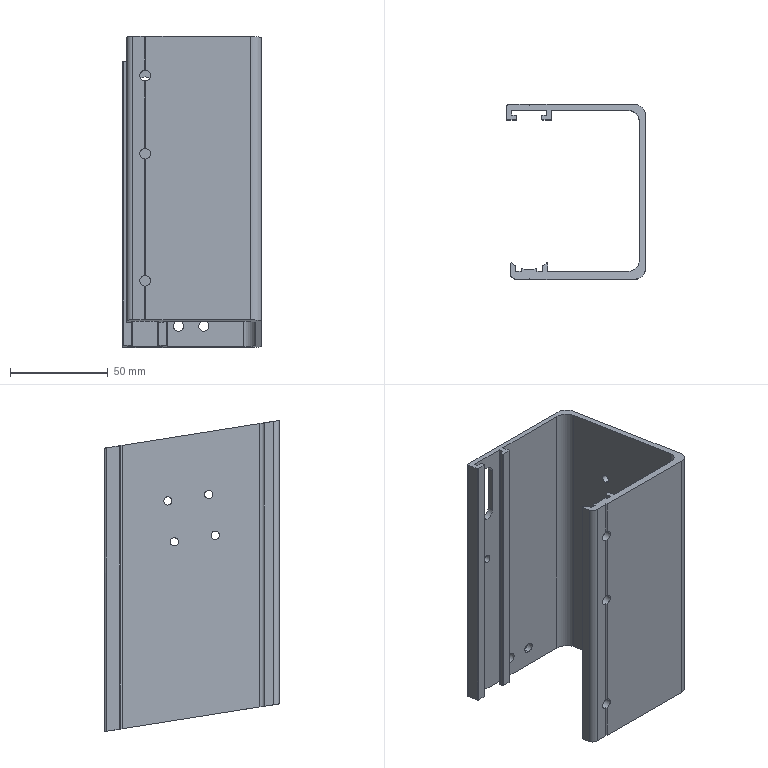Part | STEP file | 31E-01002XJ16 | 1 solid | 90 faces | box 71 x 89.5 x 159.175 mm | volume 114683 mm3 | cylinder 45 | plane 45 | commonest cylinder face diameters 1 x10 4.2 x10 5.5 x6 5.2 x4 8 x4 25.4 x3